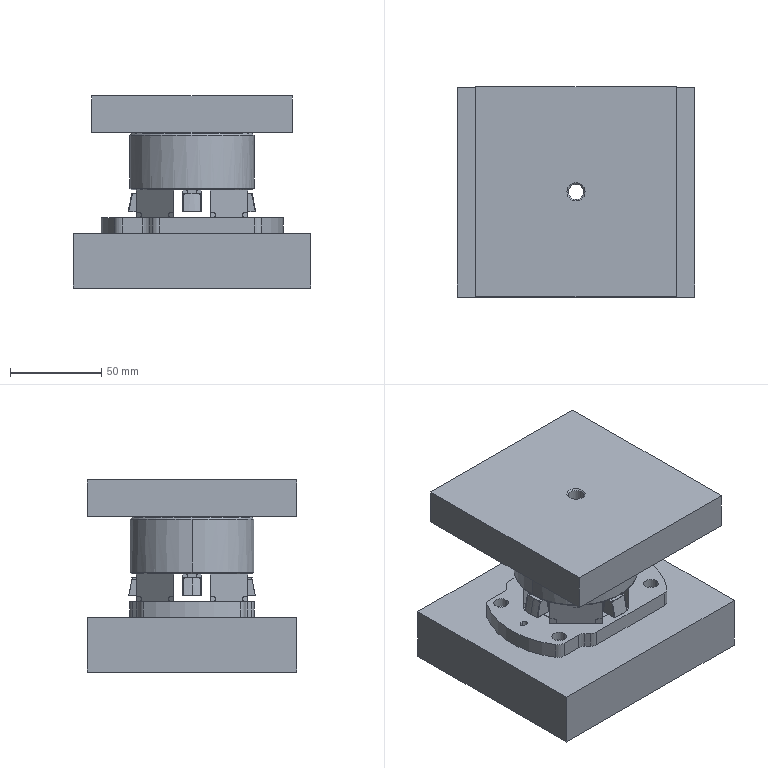NC program | NX | posted with a generic post | part box 130 x 115 x 105.2 mm
Lines 2817 to 3709 of 3709:
(113 , TOOL : ER25-D4-32_G)
N5614 T12 M6
N5616 G54
N5618 G17 G0 G90 X2.997 Y23.75 B0. C0. S3500 M3
N5620 G43 Z105.2 H12
N5622 G94 G1 Z50.2 F4500.
N5624 G41 X3. Y27.55 F500. D12
N5626 Y27.642 F458.
N5628 Y27.733 F417.
N5630 Y27.825 F375.
N5632 Y27.917 F333.
N5634 Y28.008 F292.
N5636 Y28.1 F250.
N5638 X2.467
N5640 X1.933 F333.
N5642 X1.4 F417.
N5644 X0.2 F500.
N5646 X-0.333 F458.
N5648 X-0.867 F417.
N5650 X-1.4 F375.
N5652 X-1.933 F333.
N5654 X-2.467 F292.
N5656 X-3. F250.
N5658 Y27.55
N5660 Y23.95 F500.
N5662 G40
N5664 X-2.997 Y23.75
N5666 X2.997 F6000.
N5668 G41 X3. Y27.55 F500.
N5670 Y27.642 F458.
N5672 Y27.733 F417.
N5674 Y27.825 F375.
N5676 Y27.917 F333.
N5678 Y28.008 F292.
N5680 Y28.1 F250.
N5682 X2.467
N5684 X1.933 F333.
N5686 X1.4 F417.
N5688 X0.2 F500.
N5690 X-0.333 F458.
N5692 X-0.867 F417.
N5694 X-1.4 F375.
N5696 X-1.933 F333.
N5698 X-2.467 F292.
N5700 X-3. F250.
N5702 Y27.55
N5704 Y23.95 F500.
N5706 G40
N5708 X-2.997 Y23.75
N5710 X2.997 F6000.
N5712 G41 X3. Y27.55 F500.
N5714 Y27.642 F458.
N5716 Y27.733 F417.
N5718 Y27.825 F375.
N5720 Y27.917 F333.
N5722 Y28.008 F292.
N5724 Y28.1 F250.
N5726 X2.467
N5728 X1.933 F333.
N5730 X1.4 F417.
N5732 X0.2 F500.
N5734 X-0.333 F458.
N5736 X-0.867 F417.
N5738 X-1.4 F375.
N5740 X-1.933 F333.
N5742 X-2.467 F292.
N5744 X-3. F250.
N5746 Y27.55
N5748 Y23.95 F500.
N5750 G40
N5752 X-2.997 Y23.75
N5754 X2.997 Z45.2 F6000.
N5756 G41 X3. Y27.55 F500.
N5758 Y27.642 F458.
N5760 Y27.733 F417.
N5762 Y27.825 F375.
N5764 Y27.917 F333.
N5766 Y28.008 F292.
N5768 Y28.1 F250.
N5770 X2.467
N5772 X1.933 F333.
N5774 X1.4 F417.
N5776 X0.2 F500.
N5778 X-0.333 F458.
N5780 X-0.867 F417.
N5782 X-1.4 F375.
N5784 X-1.933 F333.
N5786 X-2.467 F292.
N5788 X-3. F250.
N5790 Y27.55
N5792 Y23.95 F500.
N5794 G40
N5796 X-2.997 Y23.75
N5798 X2.997 F6000.
N5800 G41 X3. Y27.55 F500.
N5802 Y27.642 F458.
N5804 Y27.733 F417.
N5806 Y27.825 F375.
N5808 Y27.917 F333.
N5810 Y28.008 F292.
N5812 Y28.1 F250.
N5814 X2.467
N5816 X1.933 F333.
N5818 X1.4 F417.
N5820 X0.2 F500.
N5822 X-0.333 F458.
N5824 X-0.867 F417.
N5826 X-1.4 F375.
N5828 X-1.933 F333.
N5830 X-2.467 F292.
N5832 X-3. F250.
N5834 Y27.55
N5836 Y23.95 F500.
N5838 G40
N5840 X-2.997 Y23.75
N5842 X2.997 F6000.
N5844 G41 X3. Y27.55 F500.
N5846 Y27.642 F458.
N5848 Y27.733 F417.
N5850 Y27.825 F375.
N5852 Y27.917 F333.
N5854 Y28.008 F292.
N5856 Y28.1 F250.
N5858 X2.467
N5860 X1.933 F333.
N5862 X1.4 F417.
N5864 X0.2 F500.
N5866 X-0.333 F458.
N5868 X-0.867 F417.
N5870 X-1.4 F375.
N5872 X-1.933 F333.
N5874 X-2.467 F292.
N5876 X-3. F250.
N5878 Y27.55
N5880 Y23.95 F500.
N5882 G40
N5884 X-2.997 Y23.75
N5886 X2.997 Z40.2 F6000.
N5888 G41 X3. Y27.55 F500.
N5890 Y27.642 F458.
N5892 Y27.733 F417.
N5894 Y27.825 F375.
N5896 Y27.917 F333.
N5898 Y28.008 F292.
N5900 Y28.1 F250.
N5902 X2.467
N5904 X1.933 F333.
N5906 X1.4 F417.
N5908 X0.2 F500.
N5910 X-0.333 F458.
N5912 X-0.867 F417.
N5914 X-1.4 F375.
N5916 X-1.933 F333.
N5918 X-2.467 F292.
N5920 X-3. F250.
N5922 Y27.55
N5924 Y23.95 F500.
N5926 G40
N5928 X-2.997 Y23.75
N5930 X2.997 F6000.
N5932 G41 X3. Y27.55 F500.
N5934 Y27.642 F458.
N5936 Y27.733 F417.
N5938 Y27.825 F375.
N5940 Y27.917 F333.
N5942 Y28.008 F292.
N5944 Y28.1 F250.
N5946 X2.467
N5948 X1.933 F333.
N5950 X1.4 F417.
N5952 X0.2 F500.
N5954 X-0.333 F458.
N5956 X-0.867 F417.
N5958 X-1.4 F375.
N5960 X-1.933 F333.
N5962 X-2.467 F292.
N5964 X-3. F250.
N5966 Y27.55
N5968 Y23.95 F500.
N5970 G40
N5972 X-2.997 Y23.75
N5974 X2.997 F6000.
N5976 G41 X3. Y27.55 F500.
N5978 Y27.642 F458.
N5980 Y27.733 F417.
N5982 Y27.825 F375.
N5984 Y27.917 F333.
N5986 Y28.008 F292.
N5988 Y28.1 F250.
N5990 X2.467
N5992 X1.933 F333.
N5994 X1.4 F417.
N5996 X0.2 F500.
N5998 X-0.333 F458.
N6000 X-0.867 F417.
N6002 X-1.4 F375.
N6004 X-1.933 F333.
N6006 X-2.467 F292.
N6008 X-3. F250.
N6010 Y27.55
N6012 Y23.95 F500.
N6014 G40
N6016 X-2.997 Y23.75
N6018 X2.997 Z35.2 F6000.
N6020 G41 X3. Y27.55 F500.
N6022 Y27.642 F458.
N6024 Y27.733 F417.
N6026 Y27.825 F375.
N6028 Y27.917 F333.
N6030 Y28.008 F292.
N6032 Y28.1 F250.
N6034 X2.467
N6036 X1.933 F333.
N6038 X1.4 F417.
N6040 X0.2 F500.
N6042 X-0.333 F458.
N6044 X-0.867 F417.
N6046 X-1.4 F375.
N6048 X-1.933 F333.
N6050 X-2.467 F292.
N6052 X-3. F250.
N6054 Y27.55
N6056 Y23.95 F500.
N6058 G40
N6060 X-2.997 Y23.75
N6062 X2.997 F6000.
N6064 G41 X3. Y27.55 F500.
N6066 Y27.642 F458.
N6068 Y27.733 F417.
N6070 Y27.825 F375.
N6072 Y27.917 F333.
N6074 Y28.008 F292.
N6076 Y28.1 F250.
N6078 X2.467
N6080 X1.933 F333.
N6082 X1.4 F417.
N6084 X0.2 F500.
N6086 X-0.333 F458.
N6088 X-0.867 F417.
N6090 X-1.4 F375.
N6092 X-1.933 F333.
N6094 X-2.467 F292.
N6096 X-3. F250.
N6098 Y27.55
N6100 Y23.95 F500.
N6102 G40
N6104 X-2.997 Y23.75
N6106 X2.997 F6000.
N6108 G41 X3. Y27.55 F500.
N6110 Y27.642 F458.
N6112 Y27.733 F417.
N6114 Y27.825 F375.
N6116 Y27.917 F333.
N6118 Y28.008 F292.
N6120 Y28.1 F250.
N6122 X2.467
N6124 X1.933 F333.
N6126 X1.4 F417.
N6128 X0.2 F500.
N6130 X-0.333 F458.
N6132 X-0.867 F417.
N6134 X-1.4 F375.
N6136 X-1.933 F333.
N6138 X-2.467 F292.
N6140 X-3. F250.
N6142 Y27.55
N6144 Y23.95 F500.
N6146 G40
N6148 X-2.997 Y23.75
N6150 X2.997 Z30.2 F6000.
N6152 G41 X3. Y27.55 F500.
N6154 Y27.642 F458.
N6156 Y27.733 F417.
N6158 Y27.825 F375.
N6160 Y27.917 F333.
N6162 Y28.008 F292.
N6164 Y28.1 F250.
N6166 X2.467
N6168 X1.933 F333.
N6170 X1.4 F417.
N6172 X0.2 F500.
N6174 X-0.333 F458.
N6176 X-0.867 F417.
N6178 X-1.4 F375.
N6180 X-1.933 F333.
N6182 X-2.467 F292.
N6184 X-3. F250.
N6186 Y27.55
N6188 Y23.95 F500.
N6190 G40
N6192 X-2.997 Y23.75
N6194 X2.997 F6000.
N6196 G41 X3. Y27.55 F500.
N6198 Y27.642 F458.
N6200 Y27.733 F417.
N6202 Y27.825 F375.
N6204 Y27.917 F333.
N6206 Y28.008 F292.
N6208 Y28.1 F250.
N6210 X2.467
N6212 X1.933 F333.
N6214 X1.4 F417.
N6216 X0.2 F500.
N6218 X-0.333 F458.
N6220 X-0.867 F417.
N6222 X-1.4 F375.
N6224 X-1.933 F333.
N6226 X-2.467 F292.
N6228 X-3. F250.
N6230 Y27.55
N6232 Y23.95 F500.
N6234 G40
N6236 X-2.997 Y23.75
N6238 X2.997 F6000.
N6240 G41 X3. Y27.55 F500.
N6242 Y27.642 F458.
N6244 Y27.733 F417.
N6246 Y27.825 F375.
N6248 Y27.917 F333.
N6250 Y28.008 F292.
N6252 Y28.1 F250.
N6254 X2.467
N6256 X1.933 F333.
N6258 X1.4 F417.
N6260 X0.2 F500.
N6262 X-0.333 F458.
N6264 X-0.867 F417.
N6266 X-1.4 F375.
N6268 X-1.933 F333.
N6270 X-2.467 F292.
N6272 X-3. F250.
N6274 Y27.55
N6276 Y23.95 F500.
N6278 G40
N6280 X-2.997 Y23.75
N6282 X2.997 Z25.3 F6000.
N6284 G41 X3. Y27.55 F500.
N6286 Y27.642 F458.
N6288 Y27.733 F417.
N6290 Y27.825 F375.
N6292 Y27.917 F333.
N6294 Y28.008 F292.
N6296 Y28.1 F250.
N6298 X2.467
N6300 X1.933 F333.
N6302 X1.4 F417.
N6304 X0.2 F500.
N6306 X-0.333 F458.
N6308 X-0.867 F417.
N6310 X-1.4 F375.
N6312 X-1.933 F333.
N6314 X-2.467 F292.
N6316 X-3. F250.
N6318 Y27.55
N6320 Y23.95 F500.
N6322 G40
N6324 X-2.997 Y23.75
N6326 X2.997 F6000.
N6328 G41 X3. Y27.55 F500.
N6330 Y27.642 F458.
N6332 Y27.733 F417.
N6334 Y27.825 F375.
N6336 Y27.917 F333.
N6338 Y28.008 F292.
N6340 Y28.1 F250.
N6342 X2.467
N6344 X1.933 F333.
N6346 X1.4 F417.
N6348 X0.2 F500.
N6350 X-0.333 F458.
N6352 X-0.867 F417.
N6354 X-1.4 F375.
N6356 X-1.933 F333.
N6358 X-2.467 F292.
N6360 X-3. F250.
N6362 Y27.55
N6364 Y23.95 F500.
N6366 G40
N6368 X-2.997 Y23.75
N6370 X2.997 F6000.
N6372 G41 X3. Y27.55 F500.
N6374 Y27.642 F458.
N6376 Y27.733 F417.
N6378 Y27.825 F375.
N6380 Y27.917 F333.
N6382 Y28.008 F292.
N6384 Y28.1 F250.
N6386 X2.467
N6388 X1.933 F333.
N6390 X1.4 F417.
N6392 X0.2 F500.
N6394 X-0.333 F458.
N6396 X-0.867 F417.
N6398 X-1.4 F375.
N6400 X-1.933 F333.
N6402 X-2.467 F292.
N6404 X-3. F250.
N6406 Y27.55
N6408 Y23.95 F500.
N6410 G40
N6412 X-2.997 Y23.75
N6414 G0 Z105.2
N6416 Y-23.75
N6418 G1 Z50.2 F4500.
N6420 G41 X-3. Y-27.55 F500.
N6422 Y-27.808 F458.
N6424 Y-28.067 F417.
N6426 Y-28.325 F375.
N6428 Y-28.583 F333.
N6430 Y-28.842 F292.
N6432 Y-29.1 F250.
N6434 X-2.467
N6436 X-1.933 F333.
N6438 X-1.4 F417.
N6440 X-0.2 F500.
N6442 X0.333 F458.
N6444 X0.867 F417.
N6446 X1.4 F375.
N6448 X1.933 F333.
N6450 X2.467 F292.
N6452 X3. F250.
N6454 Y-28.567
N6456 Y-28.033 F333.
N6458 Y-27.55 F417.
N6460 Y-23.95 F500.
N6462 G40
N6464 X2.997 Y-23.75
N6466 X-2.997 F6000.
N6468 G41 X-3. Y-27.55 F500.
N6470 Y-27.808 F458.
N6472 Y-28.067 F417.
N6474 Y-28.325 F375.
N6476 Y-28.583 F333.
N6478 Y-28.842 F292.
N6480 Y-29.1 F250.
N6482 X-2.467
N6484 X-1.933 F333.
N6486 X-1.4 F417.
N6488 X-0.2 F500.
N6490 X0.333 F458.
N6492 X0.867 F417.
N6494 X1.4 F375.
N6496 X1.933 F333.
N6498 X2.467 F292.
N6500 X3. F250.
N6502 Y-28.567
N6504 Y-28.033 F333.
N6506 Y-27.55 F417.
N6508 Y-23.95 F500.
N6510 G40
N6512 X2.997 Y-23.75
N6514 X-2.997 F6000.
N6516 G41 X-3. Y-27.55 F500.
N6518 Y-27.808 F458.
N6520 Y-28.067 F417.
N6522 Y-28.325 F375.
N6524 Y-28.583 F333.
N6526 Y-28.842 F292.
N6528 Y-29.1 F250.
N6530 X-2.467
N6532 X-1.933 F333.
N6534 X-1.4 F417.
N6536 X-0.2 F500.
N6538 X0.333 F458.
N6540 X0.867 F417.
N6542 X1.4 F375.
N6544 X1.933 F333.
N6546 X2.467 F292.
N6548 X3. F250.
N6550 Y-28.567
N6552 Y-28.033 F333.
N6554 Y-27.55 F417.
N6556 Y-23.95 F500.
N6558 G40
N6560 X2.997 Y-23.75
N6562 X-2.997 Z45.2 F6000.
N6564 G41 X-3. Y-27.55 F500.
N6566 Y-27.808 F458.
N6568 Y-28.067 F417.
N6570 Y-28.325 F375.
N6572 Y-28.583 F333.
N6574 Y-28.842 F292.
N6576 Y-29.1 F250.
N6578 X-2.467
N6580 X-1.933 F333.
N6582 X-1.4 F417.
N6584 X-0.2 F500.
N6586 X0.333 F458.
N6588 X0.867 F417.
N6590 X1.4 F375.
N6592 X1.933 F333.
N6594 X2.467 F292.
N6596 X3. F250.
N6598 Y-28.567
N6600 Y-28.033 F333.
N6602 Y-27.55 F417.
N6604 Y-23.95 F500.
N6606 G40
N6608 X2.997 Y-23.75
N6610 X-2.997 F6000.
N6612 G41 X-3. Y-27.55 F500.
N6614 Y-27.808 F458.
N6616 Y-28.067 F417.
N6618 Y-28.325 F375.
N6620 Y-28.583 F333.
N6622 Y-28.842 F292.
N6624 Y-29.1 F250.
N6626 X-2.467
N6628 X-1.933 F333.
N6630 X-1.4 F417.
N6632 X-0.2 F500.
N6634 X0.333 F458.
N6636 X0.867 F417.
N6638 X1.4 F375.
N6640 X1.933 F333.
N6642 X2.467 F292.
N6644 X3. F250.
N6646 Y-28.567
N6648 Y-28.033 F333.
N6650 Y-27.55 F417.
N6652 Y-23.95 F500.
N6654 G40
N6656 X2.997 Y-23.75
N6658 X-2.997 F6000.
N6660 G41 X-3. Y-27.55 F500.
N6662 Y-27.808 F458.
N6664 Y-28.067 F417.
N6666 Y-28.325 F375.
N6668 Y-28.583 F333.
N6670 Y-28.842 F292.
N6672 Y-29.1 F250.
N6674 X-2.467
N6676 X-1.933 F333.
N6678 X-1.4 F417.
N6680 X-0.2 F500.
N6682 X0.333 F458.
N6684 X0.867 F417.
N6686 X1.4 F375.
N6688 X1.933 F333.
N6690 X2.467 F292.
N6692 X3. F250.
N6694 Y-28.567
N6696 Y-28.033 F333.
N6698 Y-27.55 F417.
N6700 Y-23.95 F500.
N6702 G40
N6704 X2.997 Y-23.75
N6706 X-2.997 Z40.2 F6000.
N6708 G41 X-3. Y-27.55 F500.
N6710 Y-27.808 F458.
N6712 Y-28.067 F417.
N6714 Y-28.325 F375.
N6716 Y-28.583 F333.
N6718 Y-28.842 F292.
N6720 Y-29.1 F250.
N6722 X-2.467
N6724 X-1.933 F333.
N6726 X-1.4 F417.
N6728 X-0.2 F500.
N6730 X0.333 F458.
N6732 X0.867 F417.
N6734 X1.4 F375.
N6736 X1.933 F333.
N6738 X2.467 F292.
N6740 X3. F250.
N6742 Y-28.567
N6744 Y-28.033 F333.
N6746 Y-27.55 F417.
N6748 Y-23.95 F500.
N6750 G40
N6752 X2.997 Y-23.75
N6754 X-2.997 F6000.
N6756 G41 X-3. Y-27.55 F500.
N6758 Y-27.808 F458.
N6760 Y-28.067 F417.
N6762 Y-28.325 F375.
N6764 Y-28.583 F333.
N6766 Y-28.842 F292.
N6768 Y-29.1 F250.
N6770 X-2.467
N6772 X-1.933 F333.
N6774 X-1.4 F417.
N6776 X-0.2 F500.
N6778 X0.333 F458.
N6780 X0.867 F417.
N6782 X1.4 F375.
N6784 X1.933 F333.
N6786 X2.467 F292.
N6788 X3. F250.
N6790 Y-28.567
N6792 Y-28.033 F333.
N6794 Y-27.55 F417.
N6796 Y-23.95 F500.
N6798 G40
N6800 X2.997 Y-23.75
N6802 X-2.997 F6000.
N6804 G41 X-3. Y-27.55 F500.
N6806 Y-27.808 F458.
N6808 Y-28.067 F417.
N6810 Y-28.325 F375.
N6812 Y-28.583 F333.
N6814 Y-28.842 F292.
N6816 Y-29.1 F250.
N6818 X-2.467
N6820 X-1.933 F333.
N6822 X-1.4 F417.
N6824 X-0.2 F500.
N6826 X0.333 F458.
N6828 X0.867 F417.
N6830 X1.4 F375.
N6832 X1.933 F333.
N6834 X2.467 F292.
N6836 X3. F250.
N6838 Y-28.567
N6840 Y-28.033 F333.
N6842 Y-27.55 F417.
N6844 Y-23.95 F500.
N6846 G40
N6848 X2.997 Y-23.75
N6850 X-2.997 Z35.2 F6000.
N6852 G41 X-3. Y-27.55 F500.
N6854 Y-27.808 F458.
N6856 Y-28.067 F417.
N6858 Y-28.325 F375.
N6860 Y-28.583 F333.
N6862 Y-28.842 F292.
N6864 Y-29.1 F250.
N6866 X-2.467
N6868 X-1.933 F333.
N6870 X-1.4 F417.
N6872 X-0.2 F500.
N6874 X0.333 F458.
N6876 X0.867 F417.
N6878 X1.4 F375.
N6880 X1.933 F333.
N6882 X2.467 F292.
N6884 X3. F250.
N6886 Y-28.567
N6888 Y-28.033 F333.
N6890 Y-27.55 F417.
N6892 Y-23.95 F500.
N6894 G40
N6896 X2.997 Y-23.75
N6898 X-2.997 F6000.
N6900 G41 X-3. Y-27.55 F500.
N6902 Y-27.808 F458.
N6904 Y-28.067 F417.
N6906 Y-28.325 F375.
N6908 Y-28.583 F333.
N6910 Y-28.842 F292.
N6912 Y-29.1 F250.
N6914 X-2.467
N6916 X-1.933 F333.
N6918 X-1.4 F417.
N6920 X-0.2 F500.
N6922 X0.333 F458.
N6924 X0.867 F417.
N6926 X1.4 F375.
N6928 X1.933 F333.
N6930 X2.467 F292.
N6932 X3. F250.
N6934 Y-28.567
N6936 Y-28.033 F333.
N6938 Y-27.55 F417.
N6940 Y-23.95 F500.
N6942 G40
N6944 X2.997 Y-23.75
N6946 X-2.997 F6000.
N6948 G41 X-3. Y-27.55 F500.
N6950 Y-27.808 F458.
N6952 Y-28.067 F417.
N6954 Y-28.325 F375.
N6956 Y-28.583 F333.
N6958 Y-28.842 F292.
N6960 Y-29.1 F250.
N6962 X-2.467
N6964 X-1.933 F333.
N6966 X-1.4 F417.
N6968 X-0.2 F500.
N6970 X0.333 F458.
N6972 X0.867 F417.
N6974 X1.4 F375.
N6976 X1.933 F333.
N6978 X2.467 F292.
N6980 X3. F250.
N6982 Y-28.567
N6984 Y-28.033 F333.
N6986 Y-27.55 F417.
N6988 Y-23.95 F500.
N6990 G40
N6992 X2.997 Y-23.75
N6994 X-2.997 Z30.2 F6000.
N6996 G41 X-3. Y-27.55 F500.
N6998 Y-27.808 F458.
N7000 Y-28.067 F417.
N7002 Y-28.325 F375.
N7004 Y-28.583 F333.
N7006 Y-28.842 F292.
N7008 Y-29.1 F250.
N7010 X-2.467
N7012 X-1.933 F333.
N7014 X-1.4 F417.
N7016 X-0.2 F500.
N7018 X0.333 F458.
N7020 X0.867 F417.
N7022 X1.4 F375.
N7024 X1.933 F333.
N7026 X2.467 F292.
N7028 X3. F250.
N7030 Y-28.567
N7032 Y-28.033 F333.
N7034 Y-27.55 F417.
N7036 Y-23.95 F500.
N7038 G40
N7040 X2.997 Y-23.75
N7042 X-2.997 F6000.
N7044 G41 X-3. Y-27.55 F500.
N7046 Y-27.808 F458.
N7048 Y-28.067 F417.
N7050 Y-28.325 F375.
N7052 Y-28.583 F333.
N7054 Y-28.842 F292.
N7056 Y-29.1 F250.
N7058 X-2.467
N7060 X-1.933 F333.
N7062 X-1.4 F417.
N7064 X-0.2 F500.
N7066 X0.333 F458.
N7068 X0.867 F417.
N7070 X1.4 F375.
N7072 X1.933 F333.
N7074 X2.467 F292.
N7076 X3. F250.
N7078 Y-28.567
N7080 Y-28.033 F333.
N7082 Y-27.55 F417.
N7084 Y-23.95 F500.
N7086 G40
N7088 X2.997 Y-23.75
N7090 X-2.997 F6000.
N7092 G41 X-3. Y-27.55 F500.
N7094 Y-27.808 F458.
N7096 Y-28.067 F417.
N7098 Y-28.325 F375.
N7100 Y-28.583 F333.
N7102 Y-28.842 F292.
N7104 Y-29.1 F250.
N7106 X-2.467
N7108 X-1.933 F333.
N7110 X-1.4 F417.
N7112 X-0.2 F500.
N7114 X0.333 F458.
N7116 X0.867 F417.
N7118 X1.4 F375.
N7120 X1.933 F333.
N7122 X2.467 F292.
N7124 X3. F250.
N7126 Y-28.567
N7128 Y-28.033 F333.
N7130 Y-27.55 F417.
N7132 Y-23.95 F500.
N7134 G40
N7136 X2.997 Y-23.75
N7138 X-2.997 Z25.3 F6000.
N7140 G41 X-3. Y-27.55 F500.
N7142 Y-27.808 F458.
N7144 Y-28.067 F417.
N7146 Y-28.325 F375.
N7148 Y-28.583 F333.
N7150 Y-28.842 F292.
N7152 Y-29.1 F250.
N7154 X-2.467
N7156 X-1.933 F333.
N7158 X-1.4 F417.
N7160 X-0.2 F500.
N7162 X0.333 F458.
N7164 X0.867 F417.
N7166 X1.4 F375.
N7168 X1.933 F333.
N7170 X2.467 F292.
N7172 X3. F250.
N7174 Y-28.567
N7176 Y-28.033 F333.
N7178 Y-27.55 F417.
N7180 Y-23.95 F500.
N7182 G40
N7184 X2.997 Y-23.75
N7186 X-2.997 F6000.
N7188 G41 X-3. Y-27.55 F500.
N7190 Y-27.808 F458.
N7192 Y-28.067 F417.
N7194 Y-28.325 F375.
N7196 Y-28.583 F333.
N7198 Y-28.842 F292.
N7200 Y-29.1 F250.
N7202 X-2.467
N7204 X-1.933 F333.
N7206 X-1.4 F417.
N7208 X-0.2 F500.
N7210 X0.333 F458.
N7212 X0.867 F417.
N7214 X1.4 F375.
N7216 X1.933 F333.
N7218 X2.467 F292.
N7220 X3. F250.
N7222 Y-28.567
N7224 Y-28.033 F333.
N7226 Y-27.55 F417.
N7228 Y-23.95 F500.
N7230 G40
N7232 X2.997 Y-23.75
N7234 X-2.997 F6000.
N7236 G41 X-3. Y-27.55 F500.
N7238 Y-27.808 F458.
N7240 Y-28.067 F417.
N7242 Y-28.325 F375.
N7244 Y-28.583 F333.
N7246 Y-28.842 F292.
N7248 Y-29.1 F250.
N7250 X-2.467
N7252 X-1.933 F333.
N7254 X-1.4 F417.
N7256 X-0.2 F500.
N7258 X0.333 F458.
N7260 X0.867 F417.
N7262 X1.4 F375.
N7264 X1.933 F333.
N7266 X2.467 F292.
N7268 X3. F250.
N7270 Y-28.567
N7272 Y-28.033 F333.
N7274 Y-27.55 F417.
N7276 Y-23.95 F500.
N7278 G40
N7280 X2.997 Y-23.75
N7282 G0 Z105.2
N7284 M5
(PLANAR_MILL , TOOL : Φ10_CHAMFER)
N7286 T02 M6
N7288 G54
N7290 G17 G0 G90 X-22.42 Y1.913 B0. C0. S3500 M3
N7292 G43 Z105.2 H2
N7294 Z55.7
N7296 G94 G1 Z53.7 F1000.
N7298 G41 X-22.913 Y2. D2
N7300 X-23.
N7302 G3 X-25. Y0. R2.
N7304 X0. Y-25. R25.
N7306 X-25. Y0. R-25.
N7308 X-22.913 Y-2. R2.002
N7310 G40
N7312 G1 X-22.42 Y-1.913
N7314 Z55.7
N7316 G0 Z105.2
(PLANAR_MILL_COPY , TOOL : Φ10_CHAMFER)
N7318 X3.913 Y21.549
N7320 Z56.2
N7322 G1 Z54.2 F600.
N7324 G41 X4. Y22.042
N7326 Y27.042
N7328 Y28.1
N7330 G3 X3. Y29.1 R1.
N7332 G1 X-3.
N7334 G3 X-4. Y28.1 R1.
N7336 G1 Y27.042
N7338 Y22.042
N7340 G40
N7342 X-3.913 Y21.549
N7344 Z56.2
N7346 G0 Z105.2
N7348 Y-22.058
N7350 Z56.2
N7352 G1 Z54.2
N7354 G41 X-4. Y-22.55
N7356 Y-27.55
N7358 Y-29.1
N7360 G3 X-3. Y-30.1 R1.
N7362 G1 X3.
N7364 G3 X4. Y-29.1 R1.
N7366 G1 Y-27.55
N7368 Y-22.55
N7370 G40
N7372 X3.913 Y-22.058
N7374 Z56.2
N7376 G0 Z105.2
N7378 M5
N7380 M2